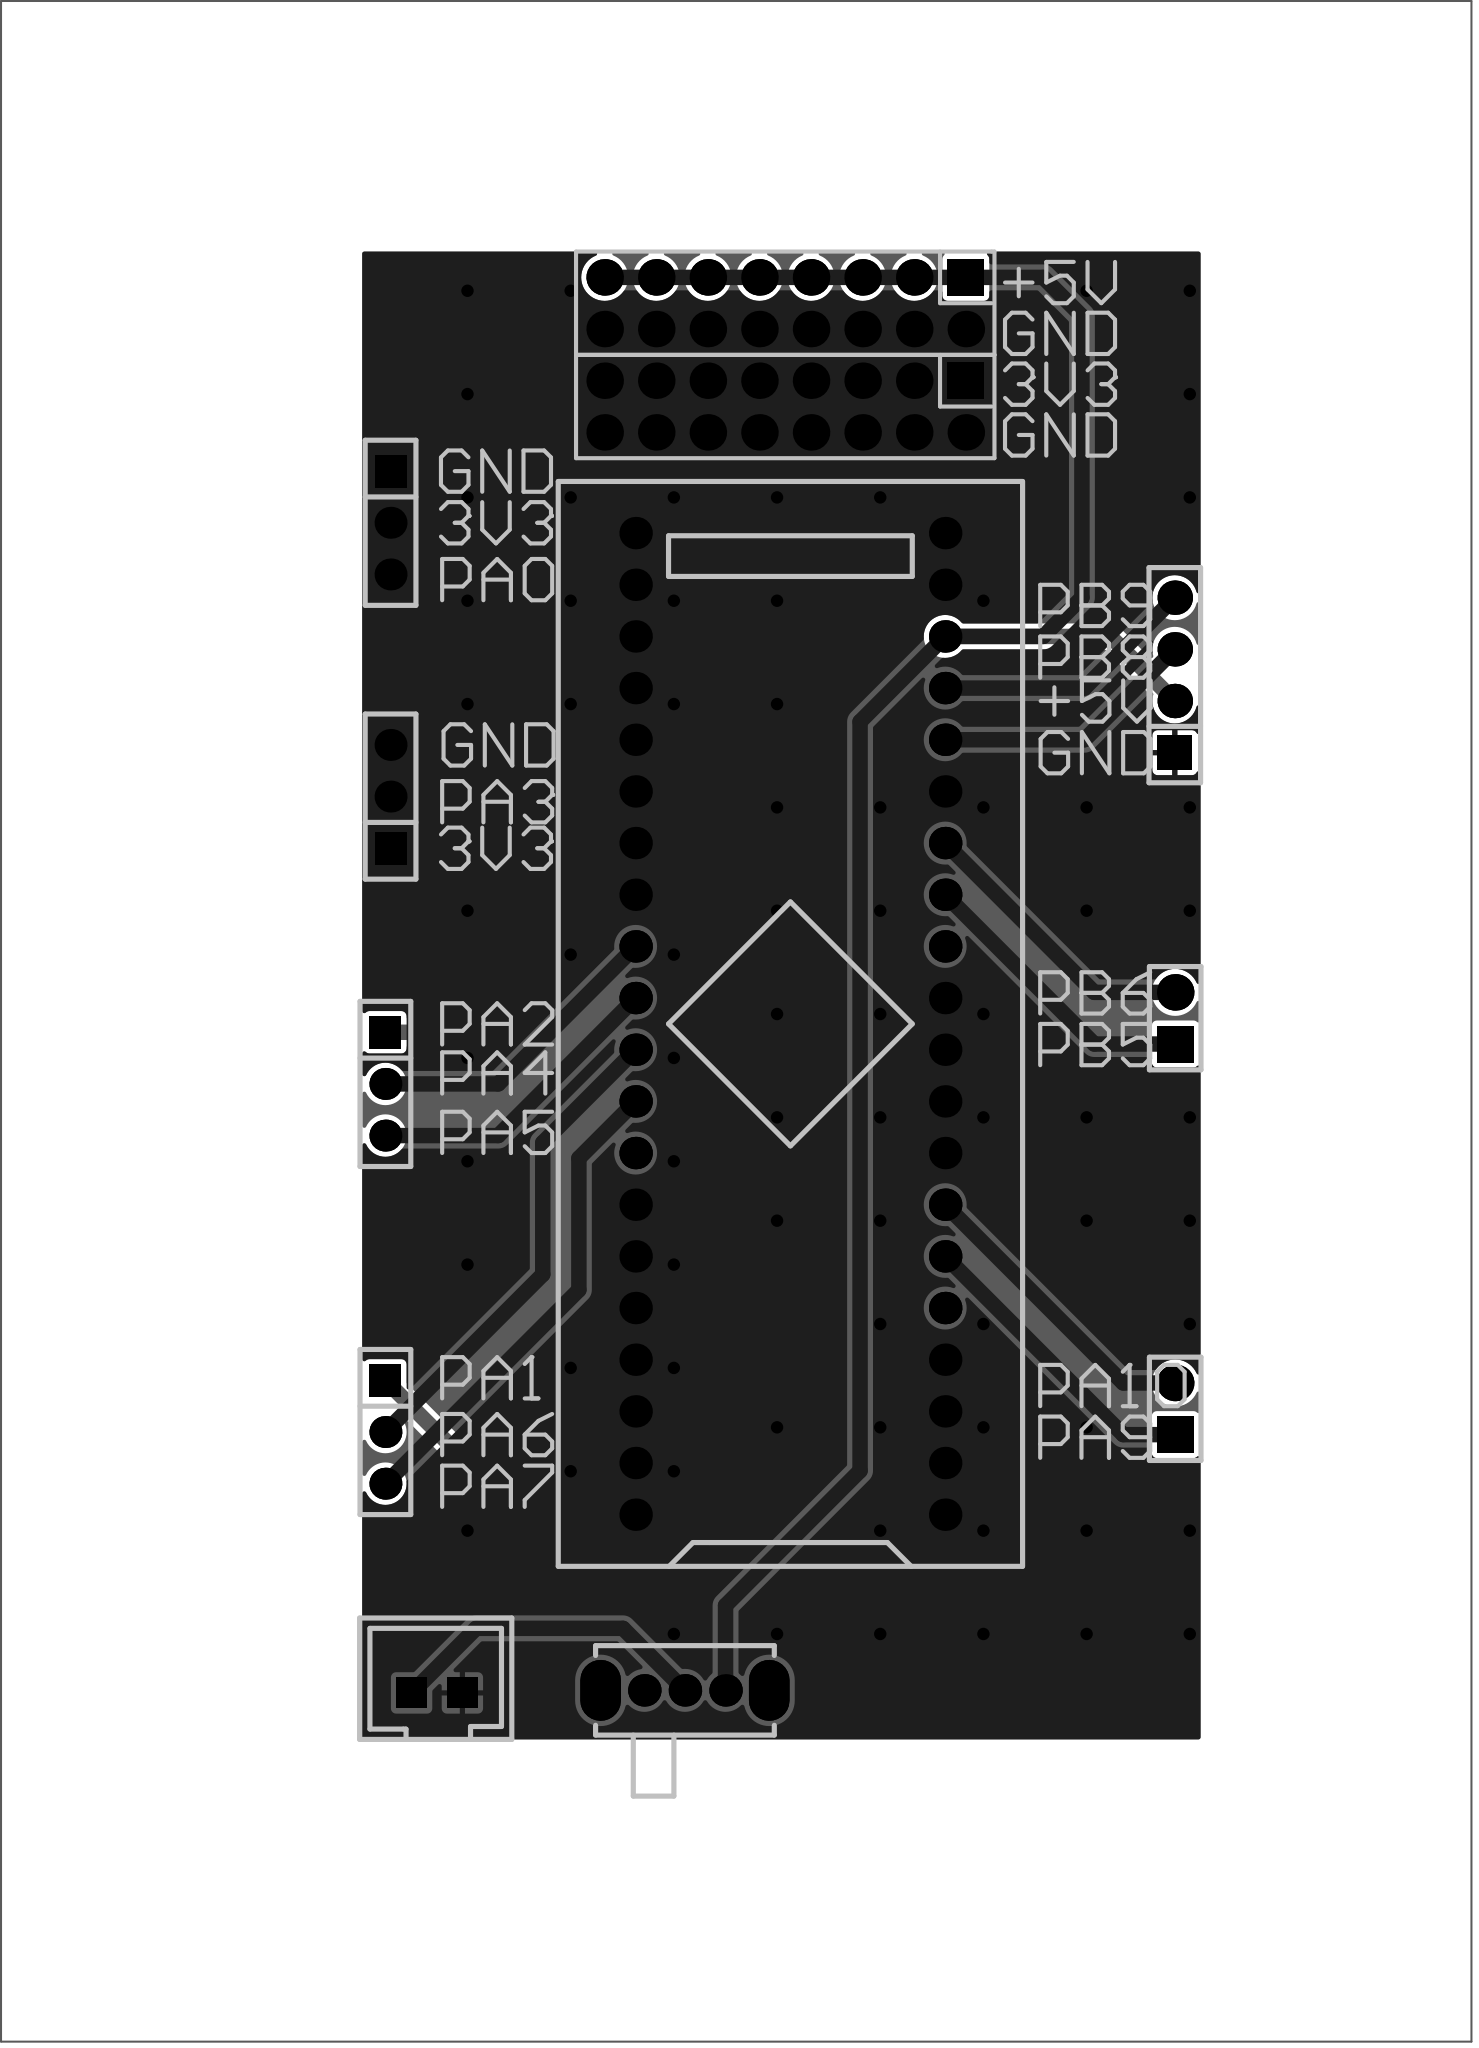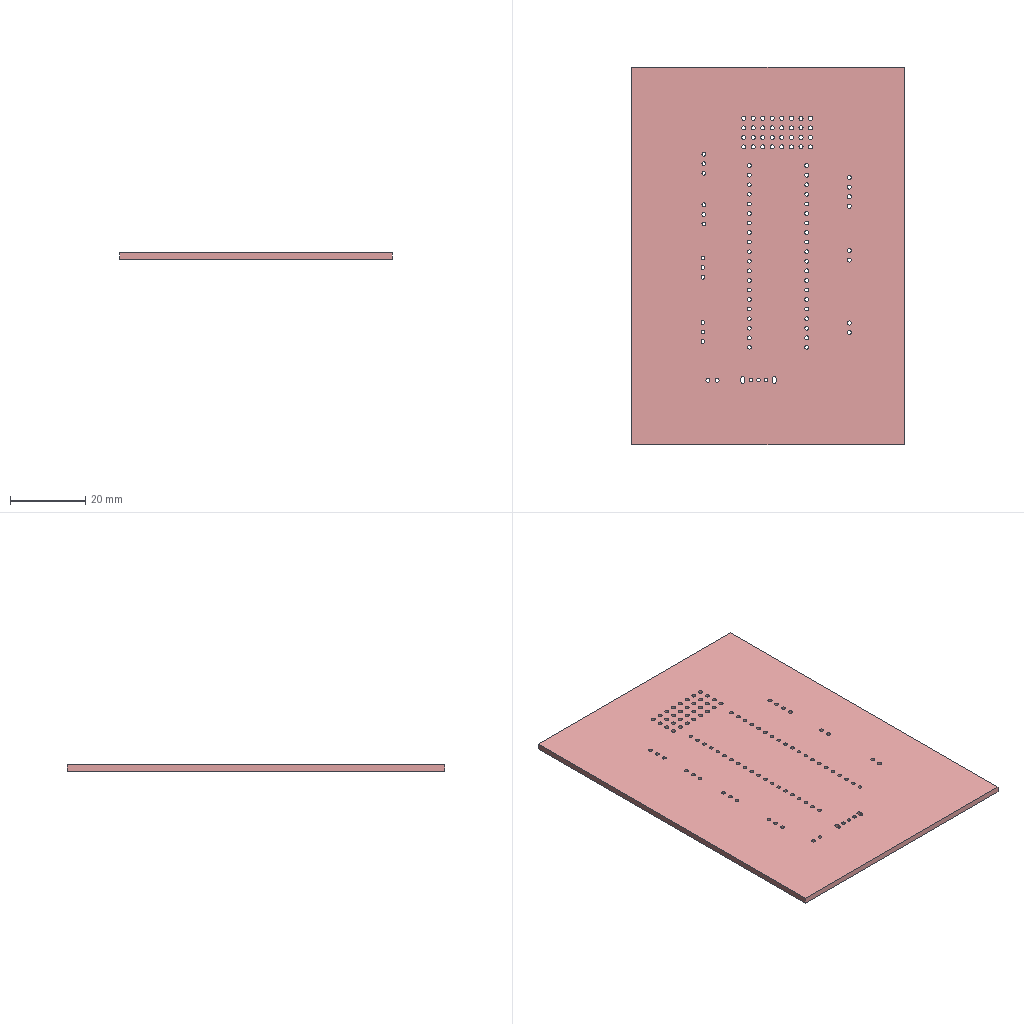Circuit board layout | Altium Designer | box 72.4 x 100.3 x 1.6 mm
Layer stack:
# Altium Designer layer stack of  (unit mm; dielectric type: 0 none, 1 core, 2 prepreg, 3 surface material)
index,name,kind,layer,copper_thickness_mm,dielectric_type,dielectric_thickness_mm,dielectric_material,dielectric_constant
0,Top Paste Mask Layer,other,,,,,,
1,Top Silkscreen Layer,other,,,,,,
2,Top Solder Mask Layer,dielectric,,,3,0.01,,3.3
3,Top Layer,copper,Top Layer,0.035,,,,
4,Dielectric1,dielectric,,,3,1.51,FR4,4.5
5,Bottom Layer,copper,Bottom Layer,0.035,,,,
6,Bottom Solder Mask Layer,dielectric,,,3,0.01,,3.3
7,Bottom Silkscreen Layer,other,,,,,,
8,Bottom Paste Mask Layer,other,,,,,,
# drill layer pairs: low layer,high layer
drill_pair,Top Layer,Bottom Layer
Part placement:
Designator,Comment,Layer,Footprint,Center-X(mm),Center-Y(mm),Rotation
U1,STM32F103C8T6-Card,TopLayer,CONN-TH_L53.3-W22.9_STM32F103C8T6-CARD,108.712,119.888,90
H1,,TopLayer,HDR-TH_16P-P2.54-V-F-R2-C8-S2.54-1,108.458,150.241,180
H2,,TopLayer,HDR-TH_16P-P2.54-V-F-R2-C8-S2.54-1,108.458,155.321,180
H6,,TopLayer,HDR-TH_3P-P2.54-V-F,88.773,99.822,270
H7,,TopLayer,HDR-TH_3P-P2.54-V-F,88.773,116.937,270
H8,,TopLayer,HDR-TH_2P-P2.54-V-M-1,127.655,100.963,90
H9,,TopLayer,HDR-TH_2P-P2.54-V-M-1,127.655,120.168,90
P1,XH2.54直插座-2P,TopLayer,CONN-TH_XH2.54-2P,91.313,86.995,0
SW1,,TopLayer,拨动开关_侧,103.519,87.121,0
H3,,TopLayer,HDR-TH_4P-P2.54-V-F,127.635,137.033,90
H4,,TopLayer,HDR-TH_3P-P2.54-V-F,89.027,144.526,270
H5,,TopLayer,HDR-TH_3P-P2.54-V-F,89.027,131.064,90
Pad and via stacks:
# Altium Designer via and pad stacks of  (unit mm). Each distinct definition once, with the count of objects using it.
# via: kind,start_layer,end_layer,hole_mm,diameter_mm,mode(0 simple;1 top-mid-bottom;2 full stack),diameter_per_layer,count,example_net
# pad: kind,layer,hole_mm,hole_type(0 round;1 square;2 slot),plating,top_size,top_shape(1 round;2 rect;3 octagon;9 rounded rect),mid_size,bottom_size,mode,footprint,size_per_layer,count,example
pad,Multi-Layer,1,0,plated,1.6x1.6,1,1.6x1.6,1.6x1.6,0,CONN-TH_L53.3-W22.9_STM32F103C8T6-CARD,,40,U1.1
pad,Multi-Layer,1.1,0,plated,1.8x1.8,1,1.8x1.8,1.8x1.8,0,HDR-TH_16P-P2.54-V-F-R2-C8-S2.54-1,,30,H1.16
pad,Multi-Layer,1.1,0,plated,1.8x1.8,2,1.8x1.8,1.8x1.8,0,HDR-TH_16P-P2.54-V-F-R2-C8-S2.54-1,,2,H1.1
pad,Multi-Layer,1.02,0,plated,1.575x1.575,1,1.575x1.575,1.575x1.575,0,HDR-TH_3P-P2.54-V-F,,8,H6.3
pad,Multi-Layer,1.02,0,plated,1.575x1.575,2,1.575x1.575,1.575x1.575,0,HDR-TH_3P-P2.54-V-F,,4,H6.1
pad,Multi-Layer,1.1,0,plated,1.8x1.8,1,1.8x1.8,1.8x1.8,0,HDR-TH_2P-P2.54-V-M-1,,2,H8.2
pad,Multi-Layer,1.1,0,plated,1.8x1.8,2,1.8x1.8,1.8x1.8,0,HDR-TH_2P-P2.54-V-M-1,,2,H8.1
pad,Multi-Layer,1,2,plated,1.524x1.524,2,1.524x1.524,1.524x1.524,0,CONN-TH_XH2.54-2P,,2,P1.1
pad,Multi-Layer,1.001,0,plated,1.6x1.6,1,1.6x1.6,1.6x1.6,0,\u00B2\u00A6\u00B6\u00AF\u00BF\u00AA\u00B9\u00D8_\u00B2\u00E0,,3,SW1.1
pad,Multi-Layer,1.001,2,plated,3x1.999,1,3x1.999,3x1.999,0,\u00B2\u00A6\u00B6\u00AF\u00BF\u00AA\u00B9\u00D8_\u00B2\u00E0,,2,SW1.4
pad,Multi-Layer,1.1,0,plated,1.7x1.7,2,1.7x1.7,1.7x1.7,0,HDR-TH_4P-P2.54-V-F,,1,H3.1
pad,Multi-Layer,1.1,0,plated,1.7x1.7,1,1.7x1.7,1.7x1.7,0,HDR-TH_4P-P2.54-V-F,,3,H3.2
via,Top Layer,Bottom Layer,0.3048,0.61,0,,73,GND
Copper pours:
name,layer,net,type(0 solid;1 hatched;2 none)
Top Layer-GND,Top Layer,GND,0
Bottom Layer-GND,Bottom Layer,GND,0